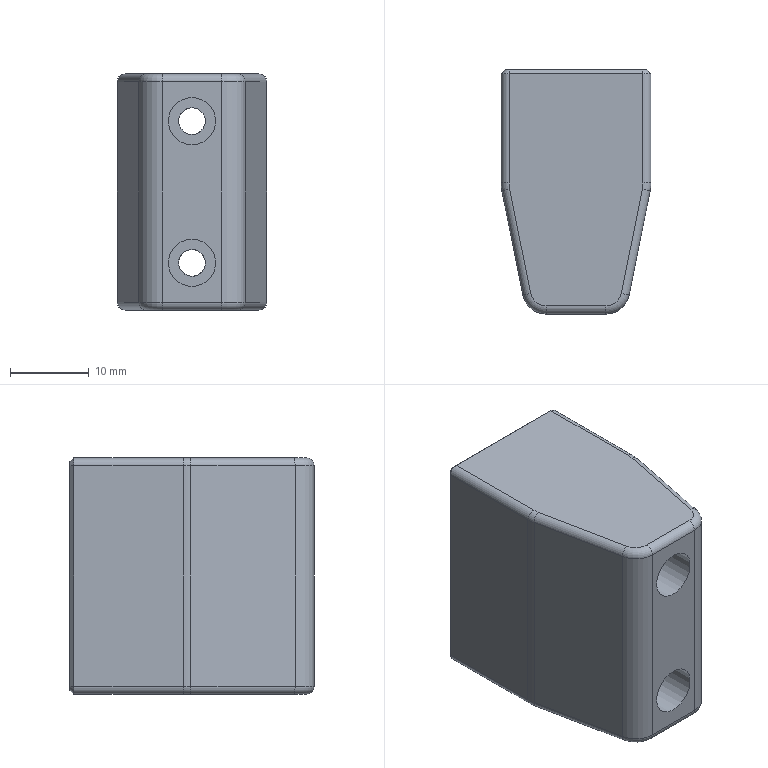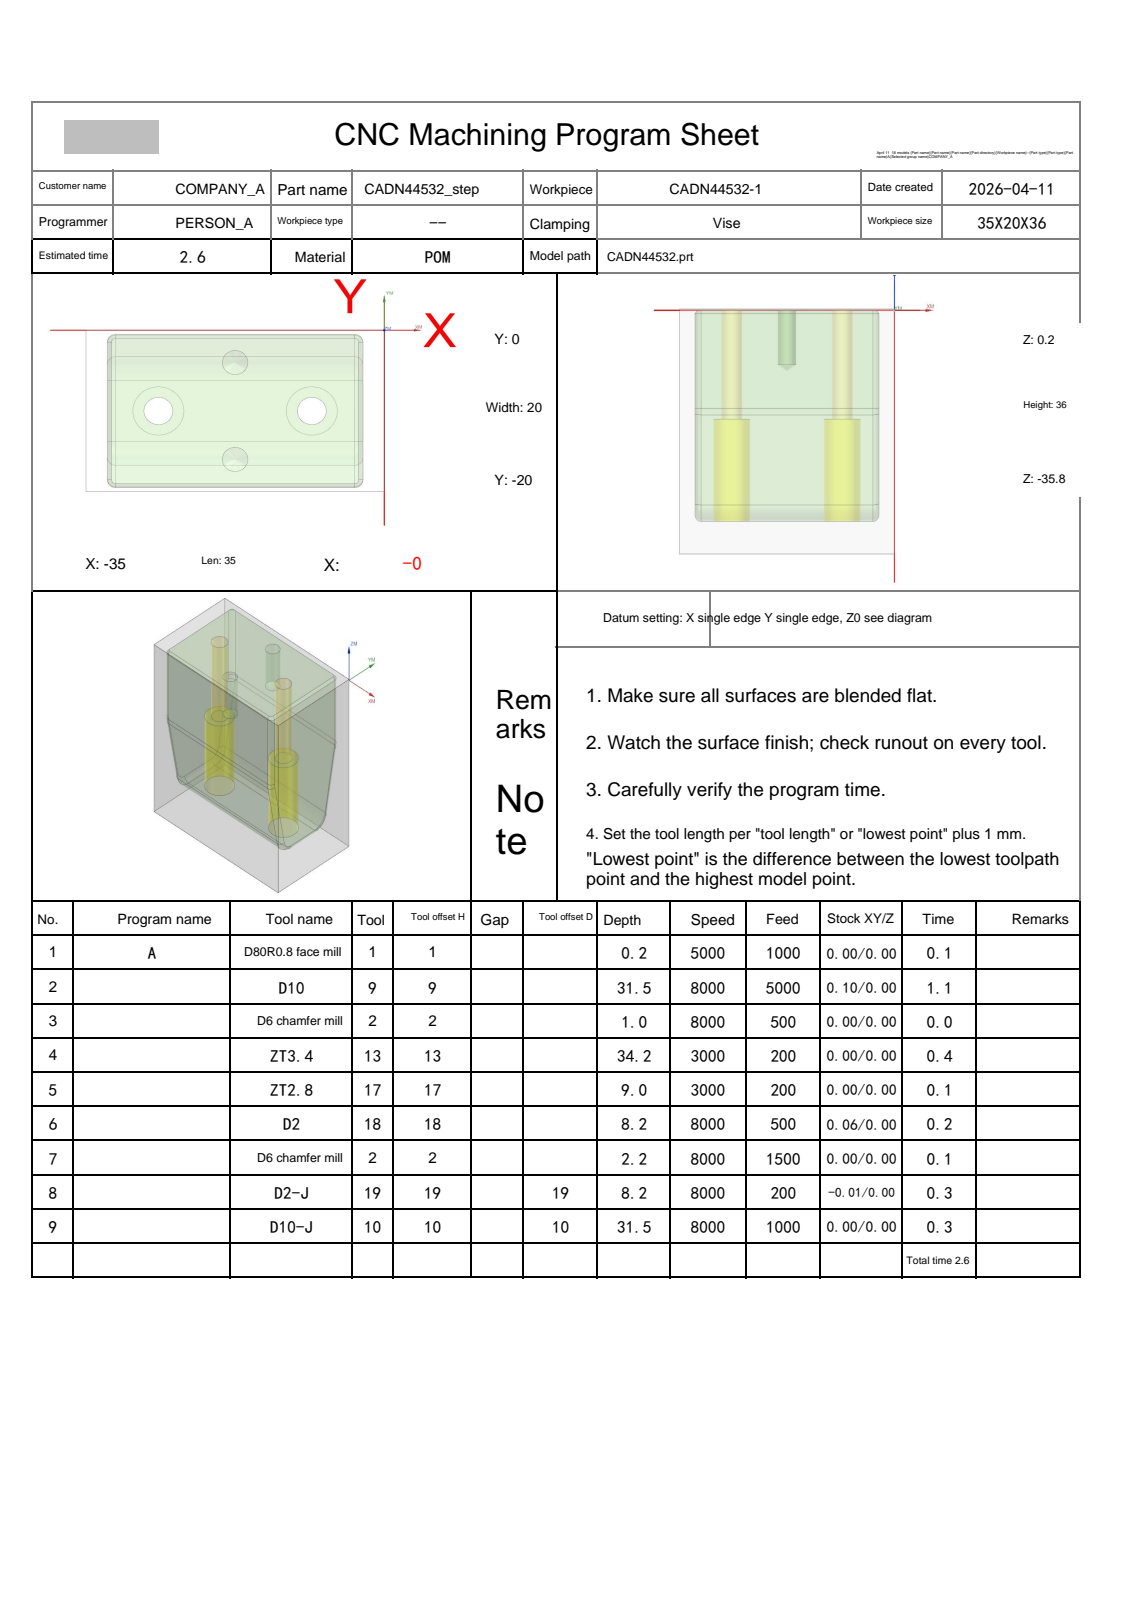NC program | NX | posted by the shop | part box 19 x 31 x 30 mm
Whole program:
%
O0001
(Machine time: 4.41 MIN)
(===Total Tool:8===)
(T1=D80R0.8 face mill D=80.  R=0.8  D-  H01 Z=0.    )
(T9=D10     D=10.  R=0.   D-  H09 Z=-31.3 )
(T2=D6 chamfer mill   D=6.   R=0.   D-  H02 Z=-2.   )
(T13=ZT3.4  D=3.4  DR_a=118 D-  H13 Z=-34.  )
(T17=ZT2.8  D=2.8  DR_a=118 D-  H17 Z=-8.8  )
(T18=D2     D=2.   R=0.   D-  H18 Z=-8.   )
(T19=D2-J   D=2.   R=0.   D19 H19 Z=-8.   )
(T10=D10-J  D=10.  R=0.   D10 H10 Z=-31.3 )
G80 G90 G17 G49 G40
G91 G28 Z0
M01
N1 T01 M06
(D80R0.8 face mill  D=80. R=0.8 H=01 ce=0.00 di=0.00)
G00 G90 G54 X-77.5 Y-10. M03 S5000
G43 H01 Z20.
M08
Z2.
G01 Z0.0 F1000.
X-72.5
X37.5
X42.5
Z2.
G00 Z20.
G91 G28 Z0.0
M05
M09
G91 G28 Z0.0
M01
N2 T09 M06
(D10  D=10. R=0. H=09 ce=0.10 di=0.00)
G00 G90 G54 X-17.5 Y-24.6 M03 S8000
G43 H09 Z20.
M08
Z.5
G01 X-31.5 Z.413 F5000.
G02 X-37.6 Y-18.5 Z.354 I0.0 J6.1
G01 Y-1.5 Z.249
G02 X-31.5 Y4.6 Z.189 I6.1 J0.0
G01 X-3.5 Z.016
G02 X2.6 Y-1.5 Z-.044 I0.0 J-6.1
G01 Y-18.421 Z-.148
G02 X-3.5 Y-24.6 Z-.208 I-6.099 J-.079
G01 X-31.5 Z-.382
G02 X-37.6 Y-18.5 Z-.441 I0.0 J6.1
G01 Y-1.5 Z-.546
G02 X-31.5 Y4.6 Z-.606 I6.1 J0.0
G01 X-3.5 Z-.779
G02 X2.6 Y-1.5 Z-.839 I0.0 J-6.1
G01 Y-18.421 Z-.943
G02 X-3.5 Y-24.6 Z-1.003 I-6.099 J-.079
G01 X-31.5 Z-1.177
G02 X-37.6 Y-18.5 Z-1.236 I0.0 J6.1
G01 Y-1.5 Z-1.341
G02 X-31.5 Y4.6 Z-1.401 I6.1 J0.0
G01 X-3.5 Z-1.574
G02 X2.6 Y-1.5 Z-1.634 I0.0 J-6.1
G01 Y-18.421 Z-1.738
G02 X-3.5 Y-24.6 Z-1.798 I-6.099 J-.079
G01 X-31.5 Z-1.972
G02 X-37.6 Y-18.5 Z-2.031 I0.0 J6.1
G01 Y-1.5 Z-2.136
G02 X-31.5 Y4.6 Z-2.196 I6.1 J0.0
G01 X-3.5 Z-2.369
G02 X2.6 Y-1.5 Z-2.429 I0.0 J-6.1
G01 Y-18.421 Z-2.533
G02 X-3.5 Y-24.6 Z-2.593 I-6.099 J-.079
G01 X-31.5 Z-2.767
G02 X-37.6 Y-18.5 Z-2.826 I0.0 J6.1
G01 Y-1.5 Z-2.931
G02 X-31.5 Y4.6 Z-2.991 I6.1 J0.0
G01 X-3.5 Z-3.164
G02 X2.6 Y-1.5 Z-3.224 I0.0 J-6.1
G01 Y-18.421 Z-3.328
G02 X-3.5 Y-24.6 Z-3.388 I-6.099 J-.079
G01 X-31.5 Z-3.562
G02 X-37.6 Y-18.5 Z-3.621 I0.0 J6.1
G01 Y-1.5 Z-3.726
G02 X-31.5 Y4.6 Z-3.786 I6.1 J0.0
G01 X-3.5 Z-3.959
G02 X2.6 Y-1.5 Z-4.019 I0.0 J-6.1
G01 Y-18.421 Z-4.123
G02 X-3.5 Y-24.6 Z-4.183 I-6.099 J-.079
G01 X-31.5 Z-4.357
G02 X-37.6 Y-18.5 Z-4.416 I0.0 J6.1
G01 Y-1.5 Z-4.521
G02 X-31.5 Y4.6 Z-4.581 I6.1 J0.0
G01 X-3.5 Z-4.754
G02 X2.6 Y-1.5 Z-4.814 I0.0 J-6.1
G01 Y-18.421 Z-4.918
G02 X-3.5 Y-24.6 Z-4.978 I-6.099 J-.079
G01 X-31.5 Z-5.152
G02 X-37.6 Y-18.5 Z-5.211 I0.0 J6.1
G01 Y-1.5 Z-5.316
G02 X-31.5 Y4.6 Z-5.376 I6.1 J0.0
G01 X-3.5 Z-5.549
G02 X2.6 Y-1.5 Z-5.609 I0.0 J-6.1
G01 Y-18.421 Z-5.713
G02 X-3.5 Y-24.6 Z-5.773 I-6.099 J-.079
G01 X-31.5 Z-5.947
G02 X-37.6 Y-18.5 Z-6.006 I0.0 J6.1
G01 Y-1.5 Z-6.111
G02 X-31.5 Y4.6 Z-6.171 I6.1 J0.0
G01 X-3.5 Z-6.344
G02 X2.6 Y-1.5 Z-6.404 I0.0 J-6.1
G01 Y-18.421 Z-6.508
G02 X-3.5 Y-24.6 Z-6.568 I-6.099 J-.079
G01 X-31.5 Z-6.742
G02 X-37.6 Y-18.5 Z-6.801 I0.0 J6.1
G01 Y-1.5 Z-6.906
G02 X-31.5 Y4.6 Z-6.966 I6.1 J0.0
G01 X-3.5 Z-7.139
G02 X2.6 Y-1.5 Z-7.199 I0.0 J-6.1
G01 Y-18.421 Z-7.303
G02 X-3.5 Y-24.6 Z-7.363 I-6.099 J-.079
G01 X-31.5 Z-7.537
G02 X-37.6 Y-18.5 Z-7.596 I0.0 J6.1
G01 Y-1.5 Z-7.701
G02 X-31.5 Y4.6 Z-7.761 I6.1 J0.0
G01 X-3.5 Z-7.934
G02 X2.6 Y-1.5 Z-7.994 I0.0 J-6.1
G01 Y-18.421 Z-8.098
G02 X-3.5 Y-24.6 Z-8.158 I-6.099 J-.079
G01 X-31.5 Z-8.332
G02 X-37.6 Y-18.5 Z-8.391 I0.0 J6.1
G01 Y-1.5 Z-8.496
G02 X-31.5 Y4.6 Z-8.556 I6.1 J0.0
G01 X-3.5 Z-8.729
G02 X2.6 Y-1.5 Z-8.789 I0.0 J-6.1
G01 Y-18.421 Z-8.893
G02 X-3.5 Y-24.6 Z-8.953 I-6.099 J-.079
G01 X-31.5 Z-9.127
G02 X-37.6 Y-18.5 Z-9.186 I0.0 J6.1
G01 Y-1.5 Z-9.291
G02 X-31.5 Y4.6 Z-9.351 I6.1 J0.0
G01 X-3.5 Z-9.524
G02 X2.6 Y-1.5 Z-9.584 I0.0 J-6.1
G01 Y-18.421 Z-9.688
G02 X-3.5 Y-24.6 Z-9.748 I-6.099 J-.079
G01 X-31.5 Z-9.922
G02 X-37.6 Y-18.5 Z-9.981 I0.0 J6.1
G01 Y-1.5 Z-10.086
G02 X-31.5 Y4.6 Z-10.146 I6.1 J0.0
G01 X-3.5 Z-10.319
G02 X2.6 Y-1.5 Z-10.379 I0.0 J-6.1
G01 Y-18.421 Z-10.483
G02 X-3.5 Y-24.6 Z-10.543 I-6.099 J-.079
G01 X-31.5 Z-10.717
G02 X-37.6 Y-18.5 Z-10.776 I0.0 J6.1
G01 Y-1.5 Z-10.881
G02 X-31.5 Y4.6 Z-10.941 I6.1 J0.0
G01 X-3.5 Z-11.114
G02 X2.6 Y-1.5 Z-11.174 I0.0 J-6.1
G01 Y-18.421 Z-11.278
G02 X-3.5 Y-24.6 Z-11.338 I-6.099 J-.079
G01 X-31.5 Z-11.512
G02 X-37.6 Y-18.5 Z-11.571 I0.0 J6.1
G01 Y-1.5 Z-11.676
G02 X-31.5 Y4.6 Z-11.736 I6.1 J0.0
G01 X-3.5 Z-11.909
G02 X2.6 Y-1.5 Z-11.969 I0.0 J-6.1
G01 Y-18.421 Z-12.073
G02 X-3.5 Y-24.6 Z-12.133 I-6.099 J-.079
G01 X-31.5 Z-12.307
G02 X-37.6 Y-18.5 Z-12.366 I0.0 J6.1
G01 Y-1.5 Z-12.471
G02 X-31.5 Y4.6 Z-12.531 I6.1 J0.0
G01 X-3.5 Z-12.704
G02 X2.6 Y-1.5 Z-12.764 I0.0 J-6.1
G01 Y-18.421 Z-12.868
G02 X-3.5 Y-24.6 Z-12.928 I-6.099 J-.079
G01 X-31.5 Z-13.102
G02 X-37.6 Y-18.5 Z-13.161 I0.0 J6.1
G01 Y-1.5 Z-13.266
G02 X-31.5 Y4.6 Z-13.326 I6.1 J0.0
G01 X-3.5 Z-13.499
G02 X2.6 Y-1.5 Z-13.559 I0.0 J-6.1
G01 Y-18.421 Z-13.663
G02 X-3.5 Y-24.6 Z-13.723 I-6.099 J-.079
G01 X-31.5 Z-13.897
G02 X-37.6 Y-18.5 Z-13.956 I0.0 J6.1
G01 Y-1.5 Z-14.061
G02 X-31.5 Y4.6 Z-14.121 I6.1 J0.0
G01 X-3.5 Z-14.294
G02 X2.6 Y-1.5 Z-14.354 I0.0 J-6.1
G01 Y-18.421 Z-14.458
G02 X-3.5 Y-24.6 Z-14.518 I-6.099 J-.079
G01 X-31.5 Z-14.692
G02 X-37.6 Y-18.5 Z-14.751 I0.0 J6.1
G01 Y-1.5 Z-14.856
G02 X-31.5 Y4.6 Z-14.916 I6.1 J0.0
G01 X-3.5 Z-15.089
G02 X2.6 Y-1.5 Z-15.149 I0.0 J-6.1
G01 Y-18.421 Z-15.253
G02 X-3.5 Y-24.6 Z-15.313 I-6.099 J-.079
G01 X-31.5 Z-15.487
G02 X-37.6 Y-18.5 Z-15.546 I0.0 J6.1
G01 Y-1.5 Z-15.651
G02 X-31.5 Y4.6 Z-15.711 I6.1 J0.0
G01 X-3.5 Z-15.884
G02 X2.6 Y-1.5 Z-15.944 I0.0 J-6.1
G01 Y-18.421 Z-16.048
G02 X-3.5 Y-24.6 Z-16.108 I-6.099 J-.079
G01 X-31.5 Z-16.282
G02 X-37.6 Y-18.5 Z-16.341 I0.0 J6.1
G01 Y-1.5 Z-16.446
G02 X-31.5 Y4.6 Z-16.506 I6.1 J0.0
G01 X-3.5 Z-16.679
G02 X2.6 Y-1.5 Z-16.739 I0.0 J-6.1
G01 Y-18.421 Z-16.843
G02 X-3.5 Y-24.6 Z-16.903 I-6.099 J-.079
G01 X-31.5 Z-17.077
G02 X-37.6 Y-18.5 Z-17.136 I0.0 J6.1
G01 Y-1.5 Z-17.241
G02 X-31.5 Y4.6 Z-17.301 I6.1 J0.0
G01 X-3.5 Z-17.474
G02 X2.6 Y-1.5 Z-17.534 I0.0 J-6.1
G01 Y-18.421 Z-17.638
G02 X-3.5 Y-24.6 Z-17.698 I-6.099 J-.079
G01 X-31.5 Z-17.872
G02 X-37.6 Y-18.5 Z-17.931 I0.0 J6.1
G01 Y-1.5 Z-18.036
G02 X-31.5 Y4.6 Z-18.096 I6.1 J0.0
G01 X-3.5 Z-18.269
G02 X2.6 Y-1.5 Z-18.329 I0.0 J-6.1
G01 Y-18.421 Z-18.433
G02 X-3.5 Y-24.6 Z-18.493 I-6.099 J-.079
G01 X-31.5 Z-18.667
G02 X-37.6 Y-18.5 Z-18.726 I0.0 J6.1
G01 Y-1.5 Z-18.831
G02 X-31.5 Y4.6 Z-18.891 I6.1 J0.0
G01 X-3.5 Z-19.064
G02 X2.6 Y-1.5 Z-19.124 I0.0 J-6.1
G01 Y-18.421 Z-19.228
G02 X-3.5 Y-24.6 Z-19.288 I-6.099 J-.079
G01 X-31.5 Z-19.462
G02 X-37.6 Y-18.5 Z-19.521 I0.0 J6.1
G01 Y-1.5 Z-19.626
G02 X-31.5 Y4.6 Z-19.686 I6.1 J0.0
G01 X-3.5 Z-19.859
G02 X2.6 Y-1.5 Z-19.919 I0.0 J-6.1
G01 Y-18.421 Z-20.023
G02 X-3.5 Y-24.6 Z-20.083 I-6.099 J-.079
G01 X-31.5 Z-20.257
G02 X-37.6 Y-18.5 Z-20.316 I0.0 J6.1
G01 Y-1.5 Z-20.421
G02 X-31.5 Y4.6 Z-20.481 I6.1 J0.0
G01 X-3.5 Z-20.654
G02 X2.6 Y-1.5 Z-20.714 I0.0 J-6.1
G01 Y-18.421 Z-20.818
G02 X-3.5 Y-24.6 Z-20.878 I-6.099 J-.079
G01 X-31.5 Z-21.052
G02 X-37.6 Y-18.5 Z-21.111 I0.0 J6.1
G01 Y-1.5 Z-21.216
G02 X-31.5 Y4.6 Z-21.276 I6.1 J0.0
G01 X-3.5 Z-21.449
G02 X2.6 Y-1.5 Z-21.509 I0.0 J-6.1
G01 Y-18.421 Z-21.613
G02 X-3.5 Y-24.6 Z-21.673 I-6.099 J-.079
G01 X-31.5 Z-21.847
G02 X-37.6 Y-18.5 Z-21.906 I0.0 J6.1
G01 Y-1.5 Z-22.011
G02 X-31.5 Y4.6 Z-22.071 I6.1 J0.0
G01 X-3.5 Z-22.244
G02 X2.6 Y-1.5 Z-22.304 I0.0 J-6.1
G01 Y-18.421 Z-22.408
G02 X-3.5 Y-24.6 Z-22.468 I-6.099 J-.079
G01 X-31.5 Z-22.642
G02 X-37.6 Y-18.5 Z-22.701 I0.0 J6.1
G01 Y-1.5 Z-22.806
G02 X-31.5 Y4.6 Z-22.866 I6.1 J0.0
G01 X-3.5 Z-23.039
G02 X2.6 Y-1.5 Z-23.099 I0.0 J-6.1
G01 Y-18.421 Z-23.203
G02 X-3.5 Y-24.6 Z-23.263 I-6.099 J-.079
G01 X-31.5 Z-23.437
G02 X-37.6 Y-18.5 Z-23.496 I0.0 J6.1
G01 Y-1.5 Z-23.601
G02 X-31.5 Y4.6 Z-23.661 I6.1 J0.0
G01 X-3.5 Z-23.834
G02 X2.6 Y-1.5 Z-23.894 I0.0 J-6.1
G01 Y-18.421 Z-23.998
G02 X-3.5 Y-24.6 Z-24.058 I-6.099 J-.079
G01 X-31.5 Z-24.232
G02 X-37.6 Y-18.5 Z-24.291 I0.0 J6.1
G01 Y-1.5 Z-24.396
G02 X-31.5 Y4.6 Z-24.456 I6.1 J0.0
G01 X-3.5 Z-24.629
G02 X2.6 Y-1.5 Z-24.689 I0.0 J-6.1
G01 Y-18.421 Z-24.793
G02 X-3.5 Y-24.6 Z-24.853 I-6.099 J-.079
G01 X-31.5 Z-25.027
G02 X-37.6 Y-18.5 Z-25.086 I0.0 J6.1
G01 Y-1.5 Z-25.191
G02 X-31.5 Y4.6 Z-25.251 I6.1 J0.0
G01 X-3.5 Z-25.424
G02 X2.6 Y-1.5 Z-25.484 I0.0 J-6.1
G01 Y-18.421 Z-25.588
G02 X-3.5 Y-24.6 Z-25.648 I-6.099 J-.079
G01 X-31.5 Z-25.822
G02 X-37.6 Y-18.5 Z-25.881 I0.0 J6.1
G01 Y-1.5 Z-25.986
G02 X-31.5 Y4.6 Z-26.046 I6.1 J0.0
G01 X-3.5 Z-26.219
G02 X2.6 Y-1.5 Z-26.279 I0.0 J-6.1
G01 Y-18.421 Z-26.383
G02 X-3.5 Y-24.6 Z-26.443 I-6.099 J-.079
G01 X-31.5 Z-26.617
G02 X-37.6 Y-18.5 Z-26.676 I0.0 J6.1
G01 Y-1.5 Z-26.781
G02 X-31.5 Y4.6 Z-26.841 I6.1 J0.0
G01 X-3.5 Z-27.014
G02 X2.6 Y-1.5 Z-27.074 I0.0 J-6.1
G01 Y-18.421 Z-27.178
G02 X-3.5 Y-24.6 Z-27.238 I-6.099 J-.079
G01 X-31.5 Z-27.412
G02 X-37.6 Y-18.5 Z-27.471 I0.0 J6.1
G01 Y-1.5 Z-27.576
G02 X-31.5 Y4.6 Z-27.636 I6.1 J0.0
G01 X-3.5 Z-27.809
G02 X2.6 Y-1.5 Z-27.869 I0.0 J-6.1
G01 Y-18.421 Z-27.973
G02 X-3.5 Y-24.6 Z-28.033 I-6.099 J-.079
G01 X-31.5 Z-28.207
G02 X-37.6 Y-18.5 Z-28.266 I0.0 J6.1
G01 Y-1.5 Z-28.371
G02 X-31.5 Y4.6 Z-28.431 I6.1 J0.0
G01 X-3.5 Z-28.604
G02 X2.6 Y-1.5 Z-28.664 I0.0 J-6.1
G01 Y-18.421 Z-28.768
G02 X-3.5 Y-24.6 Z-28.828 I-6.099 J-.079
G01 X-31.5 Z-29.002
G02 X-37.6 Y-18.5 Z-29.061 I0.0 J6.1
G01 Y-1.5 Z-29.166
G02 X-31.5 Y4.6 Z-29.226 I6.1 J0.0
G01 X-3.5 Z-29.399
G02 X2.6 Y-1.5 Z-29.459 I0.0 J-6.1
G01 Y-18.421 Z-29.563
G02 X-3.5 Y-24.6 Z-29.623 I-6.099 J-.079
G01 X-31.5 Z-29.797
G02 X-37.6 Y-18.5 Z-29.856 I0.0 J6.1
G01 Y-1.5 Z-29.961
G02 X-31.5 Y4.6 Z-30.021 I6.1 J0.0
G01 X-3.5 Z-30.194
G02 X2.6 Y-1.5 Z-30.254 I0.0 J-6.1
G01 Y-18.421 Z-30.358
G02 X-3.5 Y-24.6 Z-30.418 I-6.099 J-.079
G01 X-31.5 Z-30.592
G02 X-37.6 Y-18.5 Z-30.651 I0.0 J6.1
G01 Y-1.5 Z-30.756
G02 X-31.5 Y4.6 Z-30.816 I6.1 J0.0
G01 X-3.5 Z-30.989
G02 X2.6 Y-1.5 Z-31.049 I0.0 J-6.1
G01 Y-18.421 Z-31.153
G02 X-3.5 Y-24.6 Z-31.213 I-6.099 J-.079
G01 X-17.5 Z-31.3
X-31.5
G02 X-37.6 Y-18.5 I0.0 J6.1
G01 Y-1.5
G02 X-31.5 Y4.6 I6.1 J0.0
G01 X-3.5
G02 X2.6 Y-1.5 I0.0 J-6.1
G01 Y-18.421
X2.601 Y-18.5
G02 X-3.499 Y-24.6 I-6.1 J0.0
G01 X-17.5
X-18.
Z-30.3
G00 Z20.
G91 G28 Z0.0
M05
M09
G91 G28 Z0.0
M01
N3 T02 M06
(D6 chamfer mill  D=6. R=0. H=02 ce=0.00 di=0.00)
G00 G90 G54 X-17.5 Y-4. M03 S8000
G43 H02 Z20.
M08
G98 G81 X-17.5 Y-4. Z-.8 R1. F500.
X-26.5 Y-10.
X-17.5 Y-16.
X-8.5 Y-10.
G80
G00 Z20.
G91 G28 Z0.0
M05
M09
G91 G28 Z0.0
M01
N4 T13 M06
(ZT3.4 D=3.4 DR_a=118 H=13)
G00 G90 G54 X-26.5 Y-10. M03 S3000
G43 H13 Z20.
M08
G98 G83 X-26.5 Y-10. Z-34. R1. F200. Q3.
X-8.5
G80
G00 Z20.
G91 G28 Z0.0
M05
M09
G91 G28 Z0.0
M01
N5 T17 M06
(ZT2.8 D=2.8 DR_a=118 H=17)
G00 G90 G54 X-17.5 Y-4. M03 S3000
G43 H17 Z20.
M08
G98 G83 X-17.5 Y-4. Z-8.801 R1. F200. Q3.
Y-16.
G80
G00 Z20.
G91 G28 Z0.0
M05
M09
G91 G28 Z0.0
M01
N6 T18 M06
(D2  D=2. R=0. H=18 ce=0.06 di=0.00)
G00 G90 G54 X-17.5 Y-4. M03 S8000
G43 H18 Z20.
M08
Z.5
G03 X-17.72 Y-4.22 I0.0 J-.22 F500.
X-17.5 Y-4.44 I.22 J0.0
X-17.5 Y-4.44 Z0.0 I0.0 J.44
X-17.5 Y-4.44 Z-.5 I0.0 J.44
X-17.5 Y-4.44 Z-1. I0.0 J.44
X-17.5 Y-4.44 Z-1.5 I0.0 J.44
X-17.5 Y-4.44 Z-2. I0.0 J.44
X-17.5 Y-4.44 Z-2.5 I0.0 J.44
X-17.5 Y-4.44 Z-3. I0.0 J.44
X-17.5 Y-4.44 Z-3.5 I0.0 J.44
X-17.5 Y-4.44 Z-4. I0.0 J.44
X-17.5 Y-4.44 Z-4.5 I0.0 J.44
X-17.5 Y-4.44 Z-5. I0.0 J.44
X-17.5 Y-4.44 Z-5.5 I0.0 J.44
X-17.5 Y-4.44 Z-6. I0.0 J.44
X-17.5 Y-4.44 Z-6.5 I0.0 J.44
X-17.5 Y-4.44 Z-7. I0.0 J.44
X-17.5 Y-4.44 Z-7.5 I0.0 J.44
X-17.5 Y-4.44 Z-8. I0.0 J.44
X-17.06 Y-4. I0.0 J.44
X-17.5 Y-3.56 I-.44 J0.0
X-17.94 Y-4. I0.0 J-.44
X-17.5 Y-4.44 I.44 J0.0
X-17.28 Y-4.22 I0.0 J.22
X-17.5 Y-4. I-.22 J0.0
G00 Z20.
Y-16.
Z.5
G03 X-17.72 Y-16.22 I0.0 J-.22
X-17.5 Y-16.44 I.22 J0.0
X-17.5 Y-16.44 Z0.0 I0.0 J.44
X-17.5 Y-16.44 Z-.5 I0.0 J.44
X-17.5 Y-16.44 Z-1. I0.0 J.44
X-17.5 Y-16.44 Z-1.5 I0.0 J.44
X-17.5 Y-16.44 Z-2. I0.0 J.44
X-17.5 Y-16.44 Z-2.5 I0.0 J.44
X-17.5 Y-16.44 Z-3. I0.0 J.44
X-17.5 Y-16.44 Z-3.5 I0.0 J.44
X-17.5 Y-16.44 Z-4. I0.0 J.44
X-17.5 Y-16.44 Z-4.5 I0.0 J.44
X-17.5 Y-16.44 Z-5. I0.0 J.44
X-17.5 Y-16.44 Z-5.5 I0.0 J.44
X-17.5 Y-16.44 Z-6. I0.0 J.44
X-17.5 Y-16.44 Z-6.5 I0.0 J.44
X-17.5 Y-16.44 Z-7. I0.0 J.44
X-17.5 Y-16.44 Z-7.5 I0.0 J.44
X-17.5 Y-16.44 Z-8. I0.0 J.44
X-17.06 Y-16. I0.0 J.44
X-17.5 Y-15.56 I-.44 J0.0
X-17.94 Y-16. I0.0 J-.44
X-17.5 Y-16.44 I.44 J0.0
X-17.28 Y-16.22 I0.0 J.22
X-17.5 Y-16. I-.22 J0.0
G00 Z20.
G91 G28 Z0.0
M05
M09
G91 G28 Z0.0
M01
N7 T02 M06
(D6 chamfer mill  D=6. R=0. H=02 ce=0.00 di=0.00)
G00 G90 G54 X-17.5 Y-4. M03 S8000
G43 H02 Z20.
M08
G98 G81 X-17.5 Y-4. Z-1.8 R3. F500.
Y-16.
G80
G00 Z20.
G00 G90 X-26.5 Y-10. M03 S8000
Z20.
G98 G81 X-26.5 Y-10. Z-2. R3. F500.
X-8.5
G80
G00 Z20.
G00 G90 X-2.326 Y-21.152 M03 S6500
Z20.
Z.3
G01 Z-1.2 F1500.
G03 X-3.5 Y-20.2 I-1.174 J-.248
G01 X-31.5
G02 X-33.2 Y-18.5 I0.0 J1.7
G01 Y-1.5
G02 X-31.5 Y.2 I1.7 J0.0
G01 X-3.5
G02 X-1.8 Y-1.5 I0.0 J-1.7
G01 Y-18.5
G02 X-3.5 Y-20.2 I-1.7 J0.0
G01 X-3.9
G03 X-5.1 Y-21.4 I0.0 J-1.2
G01 Z.3
G00 Z20.
G91 G28 Z0.0
M05
M09
G91 G28 Z0.0
M01
N8 T19 M06
(D2-J  D=2. R=0. H=19 ce=-0.01 di=0.00)
G00 G90 G54 X-17.5 Y-4. M03 S8000
G43 H19 Z20.
M08
Z.5
G41 D19
G01 X-17.647 Y-4.136 F200.
X-17.716 Y-4.294
G03 X-17.5 Y-4.51 I.216 J0.0
X-17.5 Y-4.51 Z-.5 I0.0 J.51
X-17.5 Y-4.51 Z-1.5 I0.0 J.51
X-17.5 Y-4.51 Z-2.5 I0.0 J.51
X-17.5 Y-4.51 Z-3.5 I0.0 J.51
X-17.5 Y-4.51 Z-4.5 I0.0 J.51
X-17.5 Y-4.51 Z-5.5 I0.0 J.51
X-17.5 Y-4.51 Z-6.5 I0.0 J.51
X-17.5 Y-4.51 Z-7.5 I0.0 J.51
X-17.5 Y-3.49 Z-8. I0.0 J.51
X-18.01 Y-4. I0.0 J-.51
X-17.5 Y-4.51 I.51 J0.0
X-16.99 Y-4. I0.0 J.51
X-17.5 Y-3.49 I-.51 J0.0
X-17.716 Y-3.706 I0.0 J-.216
G01 X-17.647 Y-3.864
G40 X-17.5 Y-4.
G00 Z20.
Y-16.
Z.5
G41 D19
G01 X-17.647 Y-16.136
X-17.716 Y-16.294
G03 X-17.5 Y-16.51 I.216 J0.0
X-17.5 Y-16.51 Z-.5 I0.0 J.51
X-17.5 Y-16.51 Z-1.5 I0.0 J.51
X-17.5 Y-16.51 Z-2.5 I0.0 J.51
X-17.5 Y-16.51 Z-3.5 I0.0 J.51
X-17.5 Y-16.51 Z-4.5 I0.0 J.51
X-17.5 Y-16.51 Z-5.5 I0.0 J.51
X-17.5 Y-16.51 Z-6.5 I0.0 J.51
X-17.5 Y-16.51 Z-7.5 I0.0 J.51
X-17.5 Y-15.49 Z-8. I0.0 J.51
X-18.01 Y-16. I0.0 J-.51
X-17.5 Y-16.51 I.51 J0.0
X-16.99 Y-16. I0.0 J.51
X-17.5 Y-15.49 I-.51 J0.0
X-17.716 Y-15.706 I0.0 J-.216
G01 X-17.647 Y-15.864
G40 X-17.5 Y-16.
G00 Z20.
G91 G28 Z0.0
M05
M09
G91 G28 Z0.0
M01
N9 T10 M06
(D10-J  D=10. R=0. H=10 ce=0.00 di=0.00)
G00 G90 G54 X-32.512 Y5.628 M03 S8000
G43 H10 Z20.
M08
Z-15.15
G01 Z-15.65 F1000.
G41 D10
X-32.497 Y5.429
G03 X-31.5 Y4.5 I.997 J.071
G01 X-3.5
G02 X2.5 Y-1.5 I0.0 J-6.
G01 Y-18.421
X2.501 Y-18.5
G02 X-3.499 Y-24.5 I-6. J0.0
G01 X-31.5
G02 X-37.5 Y-18.5 I0.0 J6.
G01 Y-1.5
G02 X-31.5 Y4.5 I6. J0.0
G01 X-31.
G03 X-30. Y5.5 I0.0 J1.
G01 G40 Y5.7
Z-15.15
G00 Z20.
X-32.512 Y5.628
Z-30.8
G01 Z-31.3
G41 D10
X-32.497 Y5.429
G03 X-31.5 Y4.5 I.997 J.071
G01 X-3.5
G02 X2.5 Y-1.5 I0.0 J-6.
G01 Y-18.421
X2.501 Y-18.5
G02 X-3.499 Y-24.5 I-6. J0.0
G01 X-31.5
G02 X-37.5 Y-18.5 I0.0 J6.
G01 Y-1.5
G02 X-31.5 Y4.5 I6. J0.0
G01 X-31.
G03 X-30. Y5.5 I0.0 J1.
G01 G40 Y5.7
Z-30.8
G00 Z20.
M05
M09
G91 G28 Z0.0
G91 G28 Y0.0
M30
%